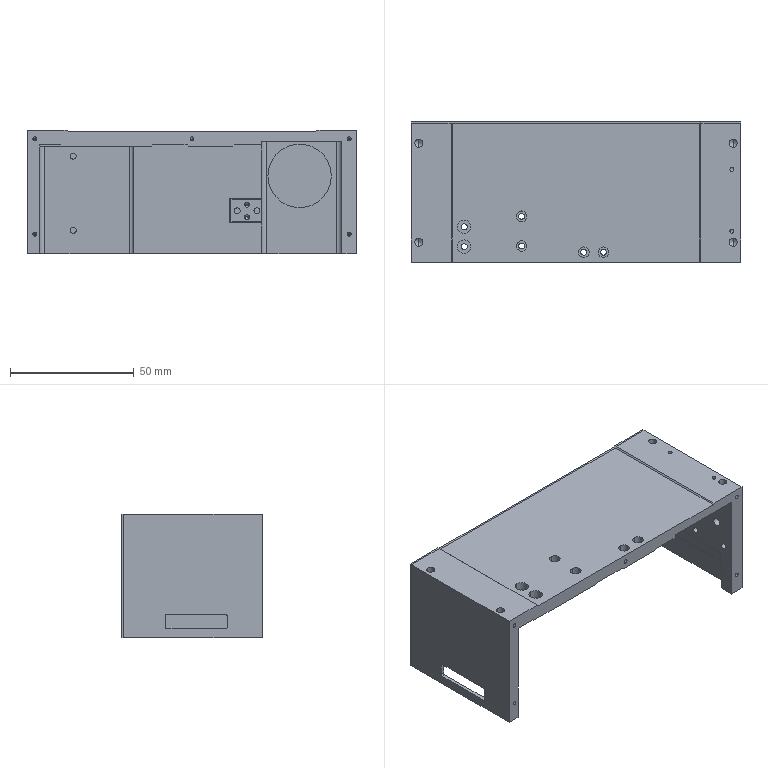NC program | NX | posted with a generic post | part box 133 x 56.74 x 50 mm
Whole program:
N10 G17 G21 G94 G90
(ZLEVEL_PROFILE_COPY , TOOL : D4)
N12 T04 M6
N14 G54
N16 G17 G0 G90 X1.724 Y-44.3 B0. C0. S9500 M3
N18 G43 Z30. H4
N20 Z1.5
N22 G94 G1 X12.07 Z0.958 F1000.
N24 Y-42.6 Z0.869
N26 X-8.53 Z-0.211
N28 Y-44.3 Z-0.3
N30 X12.07 F2000.
N32 Y-42.6
N34 X-8.53
N36 Y-44.3
N38 X8.657 Z-0.6
N40 X12.07
N42 Y-42.6
N44 X-8.53
N46 Y-44.3
N48 X8.657 Z-0.9
N50 X12.07
N52 Y-42.6
N54 X-8.53
N56 Y-44.3
N58 X8.657 Z-1.2
N60 X12.07
N62 Y-42.6
N64 X-8.53
N66 Y-44.3
N68 X8.657 Z-1.5
N70 X12.07
N72 Y-42.6
N74 X-8.53
N76 Y-44.3
N78 X8.657
N80 Z0.
N82 G0 Z30.
(ZLEVEL_PROFILE_COPY_COPY , TOOL : D4)
N84 X-8.63 Y-44.4
N86 Z3.
N88 G1 Z-1.5 F1000.
N90 X12.17
N92 Y-42.5
N94 X-8.63
N96 Y-44.4
N98 G3 X-8.284 Y-44.2 R0.4
N100 G1 Z1.5
N102 G0 Z30.
N104 M5
(ZLEVEL_PROFILE_COPY_COPY_1 , TOOL : D1)
N106 T01 M6
N108 G54
N110 G17 G0 G90 X11.925 Y-45.7 B0. C0. S9500 M3
N112 G43 Z30. H1
N114 Z0.921
N116 G94 G1 Z-0.079 F800.
N118 X12.012 Y-45.85
N120 X12.033 Y-45.913
N122 X12.098 Y-45.9
N124 X13.442
N126 X13.67 Y-45.885
N128 Y-44.328
N130 X13.683 Y-44.263
N132 X13.62 Y-44.242
N134 X13.47 Y-44.155
N136 Z0.921
N138 G0 X11.925 Y-45.7 Z0.842
N140 G1 Z-0.158
N142 X12.012 Y-45.85
N144 X12.033 Y-45.913
N146 X12.098 Y-45.9
N148 X13.442
N150 X13.67 Y-45.885
N152 Y-44.328
N154 X13.683 Y-44.263
N156 X13.62 Y-44.242
N158 X13.47 Y-44.155
N160 Z0.842
N162 G0 X11.925 Y-45.7 Z0.763
N164 G1 Z-0.237
N166 X12.012 Y-45.85
N168 X12.033 Y-45.913
N170 X12.098 Y-45.9
N172 X13.442
N174 X13.67 Y-45.885
N176 Y-44.328
N178 X13.683 Y-44.263
N180 X13.62 Y-44.242
N182 X13.47 Y-44.155
N184 Z0.763
N186 G0 X11.925 Y-45.7 Z0.684
N188 G1 Z-0.316
N190 X12.012 Y-45.85
N192 X12.033 Y-45.913
N194 X12.098 Y-45.9
N196 X13.442
N198 X13.67 Y-45.885
N200 Y-44.328
N202 X13.683 Y-44.263
N204 X13.62 Y-44.242
N206 X13.47 Y-44.155
N208 Z0.684
N210 G0 X11.925 Y-45.7 Z0.605
N212 G1 Z-0.395
N214 X12.012 Y-45.85
N216 X12.033 Y-45.913
N218 X12.098 Y-45.9
N220 X13.442
N222 X13.67 Y-45.885
N224 Y-44.328
N226 X13.683 Y-44.263
N228 X13.62 Y-44.242
N230 X13.47 Y-44.155
N232 Z0.605
N234 G0 X11.925 Y-45.7 Z0.526
N236 G1 Z-0.474
N238 X12.012 Y-45.85
N240 X12.033 Y-45.913
N242 X12.098 Y-45.9
N244 X13.442
N246 X13.67 Y-45.885
N248 Y-44.328
N250 X13.683 Y-44.263
N252 X13.62 Y-44.242
N254 X13.47 Y-44.155
N256 Z0.526
N258 G0 X11.925 Y-45.7 Z0.447
N260 G1 Z-0.553
N262 X12.012 Y-45.85
N264 X12.033 Y-45.913
N266 X12.098 Y-45.9
N268 X13.442
N270 X13.67 Y-45.885
N272 Y-44.328
N274 X13.683 Y-44.263
N276 X13.62 Y-44.242
N278 X13.47 Y-44.155
N280 Z0.447
N282 G0 X11.925 Y-45.7 Z0.368
N284 G1 Z-0.632
N286 X12.012 Y-45.85
N288 X12.033 Y-45.913
N290 X12.098 Y-45.9
N292 X13.442
N294 X13.67 Y-45.885
N296 Y-44.328
N298 X13.683 Y-44.263
N300 X13.62 Y-44.242
N302 X13.47 Y-44.155
N304 Z0.368
N306 G0 X11.925 Y-45.7 Z0.289
N308 G1 Z-0.711
N310 X12.012 Y-45.85
N312 X12.033 Y-45.913
N314 X12.098 Y-45.9
N316 X13.442
N318 X13.67 Y-45.885
N320 Y-44.328
N322 X13.683 Y-44.263
N324 X13.62 Y-44.242
N326 X13.47 Y-44.155
N328 Z0.289
N330 G0 X11.925 Y-45.7 Z0.211
N332 G1 Z-0.789
N334 X12.012 Y-45.85
N336 X12.033 Y-45.913
N338 X12.098 Y-45.9
N340 X13.442
N342 X13.67 Y-45.885
N344 Y-44.328
N346 X13.683 Y-44.263
N348 X13.62 Y-44.242
N350 X13.47 Y-44.155
N352 Z0.211
N354 G0 X11.925 Y-45.7 Z0.132
N356 G1 Z-0.868
N358 X12.012 Y-45.85
N360 X12.033 Y-45.913
N362 X12.098 Y-45.9
N364 X13.442
N366 X13.67 Y-45.885
N368 Y-44.328
N370 X13.683 Y-44.263
N372 X13.62 Y-44.242
N374 X13.47 Y-44.155
N376 Z0.132
N378 G0 X11.925 Y-45.7 Z0.053
N380 G1 Z-0.947
N382 X12.012 Y-45.85
N384 X12.033 Y-45.913
N386 X12.098 Y-45.9
N388 X13.442
N390 X13.67 Y-45.885
N392 Y-44.328
N394 X13.683 Y-44.263
N396 X13.62 Y-44.242
N398 X13.47 Y-44.155
N400 Z0.053
N402 G0 X11.925 Y-45.7 Z-0.026
N404 G1 Z-1.026
N406 X12.012 Y-45.85
N408 X12.033 Y-45.913
N410 X12.098 Y-45.9
N412 X13.442
N414 X13.67 Y-45.885
N416 Y-44.328
N418 X13.683 Y-44.263
N420 X13.62 Y-44.242
N422 X13.47 Y-44.155
N424 Z-0.026
N426 G0 X11.925 Y-45.7 Z-0.105
N428 G1 Z-1.105
N430 X12.011 Y-45.85
N432 X12.033 Y-45.913
N434 X12.098 Y-45.9
N436 X13.442
N438 X13.67 Y-45.885
N440 Y-44.328
N442 X13.683 Y-44.263
N444 X13.62 Y-44.241
N446 X13.47 Y-44.155
N448 Z-0.105
N450 G0 X11.925 Y-45.7 Z-0.184
N452 G1 Z-1.184
N454 X12.011 Y-45.85
N456 X12.033 Y-45.913
N458 X12.098 Y-45.9
N460 X13.442
N462 X13.67 Y-45.885
N464 Y-44.328
N466 X13.683 Y-44.263
N468 X13.62 Y-44.241
N470 X13.47 Y-44.155
N472 Z-0.184
N474 G0 X11.925 Y-45.7 Z-0.263
N476 G1 Z-1.263
N478 X12.011 Y-45.85
N480 X12.033 Y-45.913
N482 X12.098 Y-45.9
N484 X13.442
N486 X13.67 Y-45.885
N488 Y-44.328
N490 X13.683 Y-44.263
N492 X13.62 Y-44.241
N494 X13.47 Y-44.155
N496 Z-0.263
N498 G0 X11.925 Y-45.7 Z-0.342
N500 G1 Z-1.342
N502 X12.011 Y-45.85
N504 X12.033 Y-45.913
N506 X12.098 Y-45.9
N508 X13.659
N510 X13.67 Y-45.885
N512 Y-44.328
N514 X13.683 Y-44.263
N516 X13.62 Y-44.241
N518 X13.47 Y-44.155
N520 Z-0.342
N522 G0 X11.925 Y-45.7 Z-0.421
N524 G1 Z-1.421
N526 X12.011 Y-45.85
N528 X12.033 Y-45.913
N530 X12.098 Y-45.9
N532 X13.658
N534 X13.67 Y-45.885
N536 Y-44.328
N538 X13.683 Y-44.263
N540 X13.62 Y-44.241
N542 X13.47 Y-44.155
N544 Z-0.421
N546 G0 X11.925 Y-45.7 Z-0.5
N548 G1 Z-1.5
N550 X12.011 Y-45.85
N552 X12.033 Y-45.913
N554 X12.098 Y-45.9
N556 X13.658
N558 X13.67 Y-45.885
N560 Y-44.328
N562 X13.683 Y-44.263
N564 X13.62 Y-44.241
N566 X13.47 Y-44.155
N568 Z-0.5
N570 G0 Z30.
N572 Y-42.745
N574 Z0.921
N576 G1 Z-0.079
N578 X13.62 Y-42.658
N580 X13.683 Y-42.637
N582 X13.67 Y-42.572
N584 Y-41.
N586 X12.098
N588 X12.033 Y-40.987
N590 X12.012 Y-41.05
N592 X11.925 Y-41.2
N594 Z0.921
N596 G0 X13.47 Y-42.745 Z0.842
N598 G1 Z-0.158
N600 X13.62 Y-42.658
N602 X13.683 Y-42.637
N604 X13.67 Y-42.572
N606 Y-41.
N608 X12.098
N610 X12.033 Y-40.987
N612 X12.012 Y-41.05
N614 X11.925 Y-41.2
N616 Z0.842
N618 G0 X13.47 Y-42.745 Z0.763
N620 G1 Z-0.237
N622 X13.62 Y-42.658
N624 X13.683 Y-42.637
N626 X13.67 Y-42.572
N628 Y-41.
N630 X12.098
N632 X12.033 Y-40.987
N634 X12.012 Y-41.05
N636 X11.925 Y-41.2
N638 Z0.763
N640 G0 X13.47 Y-42.745 Z0.684
N642 G1 Z-0.316
N644 X13.62 Y-42.658
N646 X13.683 Y-42.637
N648 X13.67 Y-42.572
N650 Y-41.
N652 X12.098
N654 X12.033 Y-40.987
N656 X12.012 Y-41.05
N658 X11.925 Y-41.2
N660 Z0.684
N662 G0 X13.47 Y-42.745 Z0.605
N664 G1 Z-0.395
N666 X13.62 Y-42.658
N668 X13.683 Y-42.637
N670 X13.67 Y-42.572
N672 Y-41.
N674 X12.098
N676 X12.033 Y-40.987
N678 X12.012 Y-41.05
N680 X11.925 Y-41.2
N682 Z0.605
N684 G0 X13.47 Y-42.745 Z0.526
N686 G1 Z-0.474
N688 X13.62 Y-42.658
N690 X13.683 Y-42.637
N692 X13.67 Y-42.572
N694 Y-41.
N696 X12.098
N698 X12.033 Y-40.987
N700 X12.012 Y-41.05
N702 X11.925 Y-41.2
N704 Z0.526
N706 G0 X13.47 Y-42.745 Z0.447
N708 G1 Z-0.553
N710 X13.62 Y-42.658
N712 X13.683 Y-42.637
N714 X13.67 Y-42.572
N716 Y-41.
N718 X12.098
N720 X12.033 Y-40.987
N722 X12.012 Y-41.05
N724 X11.925 Y-41.2
N726 Z0.447
N728 G0 X13.47 Y-42.745 Z0.368
N730 G1 Z-0.632
N732 X13.62 Y-42.658
N734 X13.683 Y-42.637
N736 X13.67 Y-42.572
N738 Y-41.
N740 X12.098
N742 X12.033 Y-40.987
N744 X12.012 Y-41.05
N746 X11.925 Y-41.2
N748 Z0.368
N750 G0 X13.47 Y-42.745 Z0.289
N752 G1 Z-0.711
N754 X13.62 Y-42.658
N756 X13.683 Y-42.637
N758 X13.67 Y-42.572
N760 Y-41.
N762 X12.098
N764 X12.033 Y-40.987
N766 X12.012 Y-41.05
N768 X11.925 Y-41.2
N770 Z0.289
N772 G0 X13.47 Y-42.745 Z0.211
N774 G1 Z-0.789
N776 X13.62 Y-42.658
N778 X13.683 Y-42.637
N780 X13.67 Y-42.572
N782 Y-41.
N784 X12.098
N786 X12.033 Y-40.987
N788 X12.012 Y-41.05
N790 X11.925 Y-41.2
N792 Z0.211
N794 G0 X13.47 Y-42.745 Z0.132
N796 G1 Z-0.868
N798 X13.62 Y-42.658
N800 X13.683 Y-42.637
N802 X13.67 Y-42.572
N804 Y-41.
N806 X12.098
N808 X12.033 Y-40.987
N810 X12.012 Y-41.05
N812 X11.925 Y-41.2
N814 Z0.132
N816 G0 X13.47 Y-42.745 Z0.053
N818 G1 Z-0.947
N820 X13.62 Y-42.658
N822 X13.683 Y-42.637
N824 X13.67 Y-42.572
N826 Y-41.
N828 X12.098
N830 X12.033 Y-40.987
N832 X12.012 Y-41.05
N834 X11.925 Y-41.2
N836 Z0.053
N838 G0 X13.47 Y-42.745 Z-0.026
N840 G1 Z-1.026
N842 X13.62 Y-42.658
N844 X13.683 Y-42.637
N846 X13.67 Y-42.572
N848 Y-41.
N850 X12.098
N852 X12.033 Y-40.987
N854 X12.012 Y-41.05
N856 X11.925 Y-41.2
N858 Z-0.026
N860 G0 X13.47 Y-42.745 Z-0.105
N862 G1 Z-1.105
N864 X13.62 Y-42.658
N866 X13.683 Y-42.637
N868 X13.67 Y-42.572
N870 Y-41.
N872 X12.098
N874 X12.033 Y-40.987
N876 X12.012 Y-41.05
N878 X11.925 Y-41.2
N880 Z-0.105
N882 G0 X13.47 Y-42.745 Z-0.184
N884 G1 Z-1.184
N886 X13.62 Y-42.658
N888 X13.683 Y-42.637
N890 X13.67 Y-42.572
N892 Y-41.
N894 X12.098
N896 X12.033 Y-40.987
N898 X12.012 Y-41.05
N900 X11.925 Y-41.2
N902 Z-0.184
N904 G0 X13.47 Y-42.745 Z-0.263
N906 G1 Z-1.263
N908 X13.62 Y-42.658
N910 X13.683 Y-42.637
N912 X13.67 Y-42.572
N914 Y-41.
N916 X12.098
N918 X12.033 Y-40.987
N920 X12.012 Y-41.05
N922 X11.925 Y-41.2
N924 Z-0.263
N926 G0 X13.47 Y-42.745 Z-0.342
N928 G1 Z-1.342
N930 X13.62 Y-42.658
N932 X13.683 Y-42.637
N934 X13.67 Y-42.572
N936 Y-41.
N938 X12.098
N940 X12.033 Y-40.987
N942 X12.012 Y-41.05
N944 X11.925 Y-41.2
N946 Z-0.342
N948 G0 X13.47 Y-42.745 Z-0.421
N950 G1 Z-1.421
N952 X13.62 Y-42.658
N954 X13.683 Y-42.637
N956 X13.67 Y-42.572
N958 Y-41.
N960 X12.098
N962 X12.033 Y-40.987
N964 X12.012 Y-41.05
N966 X11.925 Y-41.2
N968 Z-0.421
N970 G0 X13.47 Y-42.745 Z-0.5
N972 G1 Z-1.5
N974 X13.62 Y-42.658
N976 X13.683 Y-42.637
N978 X13.67 Y-42.572
N980 Y-41.
N982 X12.098
N984 X12.033 Y-40.987
N986 X12.012 Y-41.05
N988 X11.925 Y-41.2
N990 Z-0.5
N992 G0 Z30.
N994 X-8.385
N996 Z0.921
N998 G1 Z-0.079
N1000 X-8.472 Y-41.05
N1002 X-8.493 Y-40.987
N1004 X-8.558 Y-41.
N1006 X-10.13
N1008 Y-42.572
N1010 X-10.143 Y-42.637
N1012 X-10.08 Y-42.658
N1014 X-9.93 Y-42.745
N1016 Z0.921
N1018 G0 X-8.385 Y-41.2 Z0.842
N1020 G1 Z-0.158
N1022 X-8.472 Y-41.05
N1024 X-8.493 Y-40.987
N1026 X-8.558 Y-41.
N1028 X-10.13
N1030 Y-42.572
N1032 X-10.143 Y-42.637
N1034 X-10.08 Y-42.658
N1036 X-9.93 Y-42.745
N1038 Z0.842
N1040 G0 X-8.385 Y-41.2 Z0.763
N1042 G1 Z-0.237
N1044 X-8.472 Y-41.05
N1046 X-8.493 Y-40.987
N1048 X-8.558 Y-41.
N1050 X-10.13
N1052 Y-42.572
N1054 X-10.143 Y-42.637
N1056 X-10.08 Y-42.658
N1058 X-9.93 Y-42.745
N1060 Z0.763
N1062 G0 X-8.385 Y-41.2 Z0.684
N1064 G1 Z-0.316
N1066 X-8.472 Y-41.05
N1068 X-8.493 Y-40.987
N1070 X-8.558 Y-41.
N1072 X-10.13
N1074 Y-42.572
N1076 X-10.143 Y-42.637
N1078 X-10.08 Y-42.658
N1080 X-9.93 Y-42.745
N1082 Z0.684
N1084 G0 X-8.385 Y-41.2 Z0.605
N1086 G1 Z-0.395
N1088 X-8.472 Y-41.05
N1090 X-8.493 Y-40.987
N1092 X-8.558 Y-41.
N1094 X-10.13
N1096 Y-42.572
N1098 X-10.143 Y-42.637
N1100 X-10.08 Y-42.658
N1102 X-9.93 Y-42.745
N1104 Z0.605
N1106 G0 X-8.385 Y-41.2 Z0.526
N1108 G1 Z-0.474
N1110 X-8.472 Y-41.05
N1112 X-8.493 Y-40.987
N1114 X-8.558 Y-41.
N1116 X-10.13
N1118 Y-42.572
N1120 X-10.143 Y-42.637
N1122 X-10.08 Y-42.658
N1124 X-9.93 Y-42.745
N1126 Z0.526
N1128 G0 X-8.385 Y-41.2 Z0.447
N1130 G1 Z-0.553
N1132 X-8.472 Y-41.05
N1134 X-8.493 Y-40.987
N1136 X-8.558 Y-41.
N1138 X-10.13
N1140 Y-42.572
N1142 X-10.143 Y-42.637
N1144 X-10.08 Y-42.658
N1146 X-9.93 Y-42.745
N1148 Z0.447
N1150 G0 X-8.385 Y-41.2 Z0.368
N1152 G1 Z-0.632
N1154 X-8.472 Y-41.05
N1156 X-8.493 Y-40.987
N1158 X-8.558 Y-41.
N1160 X-10.13
N1162 Y-42.572
N1164 X-10.143 Y-42.637
N1166 X-10.08 Y-42.658
N1168 X-9.93 Y-42.745
N1170 Z0.368
N1172 G0 X-8.385 Y-41.2 Z0.289
N1174 G1 Z-0.711
N1176 X-8.472 Y-41.05
N1178 X-8.493 Y-40.987
N1180 X-8.558 Y-41.
N1182 X-10.13
N1184 Y-42.572
N1186 X-10.143 Y-42.637
N1188 X-10.08 Y-42.658
N1190 X-9.93 Y-42.745
N1192 Z0.289
N1194 G0 X-8.385 Y-41.2 Z0.211
N1196 G1 Z-0.789
N1198 X-8.472 Y-41.05
N1200 X-8.493 Y-40.987
N1202 X-8.558 Y-41.
N1204 X-10.13
N1206 Y-42.572
N1208 X-10.143 Y-42.637
N1210 X-10.08 Y-42.658
N1212 X-9.93 Y-42.745
N1214 Z0.211
N1216 G0 X-8.385 Y-41.2 Z0.132
N1218 G1 Z-0.868
N1220 X-8.472 Y-41.05
N1222 X-8.493 Y-40.987
N1224 X-8.558 Y-41.
N1226 X-10.13
N1228 Y-42.572
N1230 X-10.143 Y-42.637
N1232 X-10.08 Y-42.658
N1234 X-9.93 Y-42.745
N1236 Z0.132
N1238 G0 X-8.385 Y-41.2 Z0.053
N1240 G1 Z-0.947
N1242 X-8.472 Y-41.05
N1244 X-8.493 Y-40.987
N1246 X-8.558 Y-41.
N1248 X-10.13
N1250 Y-42.572
N1252 X-10.143 Y-42.637
N1254 X-10.08 Y-42.658
N1256 X-9.93 Y-42.745
N1258 Z0.053
N1260 G0 X-8.385 Y-41.2 Z-0.026
N1262 G1 Z-1.026
N1264 X-8.472 Y-41.05
N1266 X-8.493 Y-40.987
N1268 X-8.558 Y-41.
N1270 X-10.13
N1272 Y-42.572
N1274 X-10.143 Y-42.637
N1276 X-10.08 Y-42.658
N1278 X-9.93 Y-42.745
N1280 Z-0.026
N1282 G0 X-8.385 Y-41.2 Z-0.105
N1284 G1 Z-1.105
N1286 X-8.472 Y-41.05
N1288 X-8.493 Y-40.987
N1290 X-8.558 Y-41.
N1292 X-10.13
N1294 Y-42.572
N1296 X-10.143 Y-42.637
N1298 X-10.08 Y-42.658
N1300 X-9.93 Y-42.745
N1302 Z-0.105
N1304 G0 X-8.385 Y-41.2 Z-0.184
N1306 G1 Z-1.184
N1308 X-8.472 Y-41.05
N1310 X-8.493 Y-40.987
N1312 X-8.558 Y-41.
N1314 X-10.13
N1316 Y-42.572
N1318 X-10.143 Y-42.637
N1320 X-10.08 Y-42.658
N1322 X-9.93 Y-42.745
N1324 Z-0.184
N1326 G0 X-8.385 Y-41.2 Z-0.263
N1328 G1 Z-1.263
N1330 X-8.472 Y-41.05
N1332 X-8.493 Y-40.987
N1334 X-8.558 Y-41.
N1336 X-10.13
N1338 Y-42.572
N1340 X-10.143 Y-42.637
N1342 X-10.08 Y-42.658
N1344 X-9.93 Y-42.745
N1346 Z-0.263
N1348 G0 X-8.385 Y-41.2 Z-0.342
N1350 G1 Z-1.342
N1352 X-8.472 Y-41.05
N1354 X-8.493 Y-40.987
N1356 X-8.558 Y-41.
N1358 X-10.13
N1360 Y-42.572
N1362 X-10.143 Y-42.637
N1364 X-10.08 Y-42.658
N1366 X-9.93 Y-42.745
N1368 Z-0.342
N1370 G0 X-8.385 Y-41.2 Z-0.421
N1372 G1 Z-1.421
N1374 X-8.472 Y-41.05
N1376 X-8.493 Y-40.987
N1378 X-8.558 Y-41.
N1380 X-10.13
N1382 Y-42.572
N1384 X-10.143 Y-42.637
N1386 X-10.08 Y-42.658
N1388 X-9.93 Y-42.745
N1390 Z-0.421
N1392 G0 X-8.385 Y-41.2 Z-0.5
N1394 G1 Z-1.5
N1396 X-8.472 Y-41.05
N1398 X-8.493 Y-40.987
N1400 X-8.558 Y-41.
N1402 X-10.129
N1404 X-10.13 Y-42.572
N1406 X-10.143 Y-42.637
N1408 X-10.08 Y-42.658
N1410 X-9.93 Y-42.745
N1412 Z-0.5
N1414 G0 Z30.
N1416 Y-44.155
N1418 Z0.921
N1420 G1 Z-0.079
N1422 X-10.08 Y-44.242
N1424 X-10.143 Y-44.263
N1426 X-10.13 Y-44.328
N1428 Y-45.9
N1430 X-8.558
N1432 X-8.493 Y-45.913
N1434 X-8.472 Y-45.85
N1436 X-8.385 Y-45.7
N1438 Z0.921
N1440 G0 X-9.93 Y-44.155 Z0.842
N1442 G1 Z-0.158
N1444 X-10.08 Y-44.242
N1446 X-10.143 Y-44.263
N1448 X-10.13 Y-44.328
N1450 Y-45.9
N1452 X-8.558
N1454 X-8.493 Y-45.913
N1456 X-8.472 Y-45.85
N1458 X-8.385 Y-45.7
N1460 Z0.842
N1462 G0 X-9.93 Y-44.155 Z0.763
N1464 G1 Z-0.237
N1466 X-10.08 Y-44.242
N1468 X-10.143 Y-44.263
N1470 X-10.13 Y-44.328
N1472 Y-45.9
N1474 X-8.558
N1476 X-8.493 Y-45.913
N1478 X-8.472 Y-45.85
N1480 X-8.385 Y-45.7
N1482 Z0.763
N1484 G0 X-9.93 Y-44.155 Z0.684
N1486 G1 Z-0.316
N1488 X-10.08 Y-44.242
N1490 X-10.143 Y-44.263
N1492 X-10.13 Y-44.328
N1494 Y-45.9
N1496 X-8.558
N1498 X-8.493 Y-45.913
N1500 X-8.472 Y-45.85
N1502 X-8.385 Y-45.7
N1504 Z0.684
N1506 G0 X-9.93 Y-44.155 Z0.605
N1508 G1 Z-0.395
N1510 X-10.08 Y-44.242
N1512 X-10.143 Y-44.263
N1514 X-10.13 Y-44.328
N1516 Y-45.9
N1518 X-8.558
N1520 X-8.493 Y-45.913
N1522 X-8.472 Y-45.85
N1524 X-8.385 Y-45.7
N1526 Z0.605
N1528 G0 X-9.93 Y-44.155 Z0.526
N1530 G1 Z-0.474
N1532 X-10.08 Y-44.242
N1534 X-10.143 Y-44.263
N1536 X-10.13 Y-44.328
N1538 Y-45.9
N1540 X-8.558
N1542 X-8.493 Y-45.913
N1544 X-8.472 Y-45.85
N1546 X-8.385 Y-45.7
N1548 Z0.526
N1550 G0 X-9.93 Y-44.155 Z0.447
N1552 G1 Z-0.553
N1554 X-10.08 Y-44.242
N1556 X-10.143 Y-44.263
N1558 X-10.13 Y-44.328
N1560 Y-45.9
N1562 X-8.558
N1564 X-8.493 Y-45.913
N1566 X-8.472 Y-45.85
N1568 X-8.385 Y-45.7
N1570 Z0.447
N1572 G0 X-9.93 Y-44.155 Z0.368
N1574 G1 Z-0.632
N1576 X-10.08 Y-44.242
N1578 X-10.143 Y-44.263
N1580 X-10.13 Y-44.328
N1582 Y-45.9
N1584 X-8.558
N1586 X-8.493 Y-45.913
N1588 X-8.472 Y-45.85
N1590 X-8.385 Y-45.7
N1592 Z0.368
N1594 G0 X-9.93 Y-44.155 Z0.289
N1596 G1 Z-0.711
N1598 X-10.08 Y-44.242
N1600 X-10.143 Y-44.263
N1602 X-10.13 Y-44.328
N1604 Y-45.9
N1606 X-8.558
N1608 X-8.493 Y-45.913
N1610 X-8.472 Y-45.85
N1612 X-8.385 Y-45.7
N1614 Z0.289
N1616 G0 X-9.93 Y-44.155 Z0.211
N1618 G1 Z-0.789
N1620 X-10.08 Y-44.242
N1622 X-10.143 Y-44.263
N1624 X-10.13 Y-44.328
N1626 Y-45.9
N1628 X-8.558
N1630 X-8.493 Y-45.913
N1632 X-8.472 Y-45.85
N1634 X-8.385 Y-45.7
N1636 Z0.211
N1638 G0 X-9.93 Y-44.155 Z0.132
N1640 G1 Z-0.868
N1642 X-10.08 Y-44.242
N1644 X-10.143 Y-44.263
N1646 X-10.13 Y-44.328
N1648 Y-45.9
N1650 X-8.558
N1652 X-8.493 Y-45.913
N1654 X-8.472 Y-45.85
N1656 X-8.385 Y-45.7
N1658 Z0.132
N1660 G0 X-9.93 Y-44.155 Z0.053
N1662 G1 Z-0.947
N1664 X-10.08 Y-44.242
N1666 X-10.143 Y-44.263
N1668 X-10.13 Y-44.328
N1670 Y-45.9
N1672 X-8.558
N1674 X-8.493 Y-45.913
N1676 X-8.472 Y-45.85
N1678 X-8.385 Y-45.7
N1680 Z0.053
N1682 G0 X-9.93 Y-44.155 Z-0.026
N1684 G1 Z-1.026
N1686 X-10.08 Y-44.242
N1688 X-10.143 Y-44.263
N1690 X-10.13 Y-44.328
N1692 Y-45.9
N1694 X-8.558
N1696 X-8.493 Y-45.913
N1698 X-8.472 Y-45.85
N1700 X-8.385 Y-45.7
N1702 Z-0.026
N1704 G0 X-9.93 Y-44.155 Z-0.105
N1706 G1 Z-1.105
N1708 X-10.08 Y-44.242
N1710 X-10.143 Y-44.263
N1712 X-10.13 Y-44.328
N1714 Y-45.9
N1716 X-8.558
N1718 X-8.493 Y-45.913
N1720 X-8.472 Y-45.85
N1722 X-8.385 Y-45.7
N1724 Z-0.105
N1726 G0 X-9.93 Y-44.155 Z-0.184
N1728 G1 Z-1.184
N1730 X-10.08 Y-44.242
N1732 X-10.143 Y-44.263
N1734 X-10.13 Y-44.328
N1736 Y-45.9
N1738 X-8.558
N1740 X-8.493 Y-45.913
N1742 X-8.472 Y-45.85
N1744 X-8.385 Y-45.7
N1746 Z-0.184
N1748 G0 X-9.93 Y-44.155 Z-0.263
N1750 G1 Z-1.263
N1752 X-10.08 Y-44.242
N1754 X-10.143 Y-44.263
N1756 X-10.13 Y-44.328
N1758 Y-45.9
N1760 X-8.558
N1762 X-8.493 Y-45.913
N1764 X-8.472 Y-45.85
N1766 X-8.385 Y-45.7
N1768 Z-0.263
N1770 G0 X-9.93 Y-44.155 Z-0.342
N1772 G1 Z-1.342
N1774 X-10.08 Y-44.242
N1776 X-10.143 Y-44.263
N1778 X-10.13 Y-44.328
N1780 Y-45.9
N1782 X-8.558
N1784 X-8.493 Y-45.913
N1786 X-8.472 Y-45.85
N1788 X-8.385 Y-45.7
N1790 Z-0.342
N1792 G0 X-9.93 Y-44.155 Z-0.421
N1794 G1 Z-1.421
N1796 X-10.08 Y-44.242
N1798 X-10.143 Y-44.263
N1800 X-10.13 Y-44.328
N1802 Y-45.9
N1804 X-8.558
N1806 X-8.493 Y-45.913
N1808 X-8.472 Y-45.85
N1810 X-8.385 Y-45.7
N1812 Z-0.421
N1814 G0 X-9.93 Y-44.155 Z-0.5
N1816 G1 Z-1.5
N1818 X-10.08 Y-44.242
N1820 X-10.143 Y-44.263
N1822 X-10.13 Y-44.328
N1824 Y-45.9
N1826 X-8.558
N1828 X-8.493 Y-45.913
N1830 X-8.472 Y-45.85
N1832 X-8.385 Y-45.7
N1834 Z-0.5
N1836 G0 Z30.
N1838 M5
(PLANAR_MILL_COPY_1_COPY , TOOL : D6A45)
N1840 T07 M6
N1842 G54
N1844 G17 G0 G90 X-8.53 Y-44.23 B0. C0. S9500 M3
N1846 G43 Z30. H7
N1848 Z0.5
N1850 G94 G1 Z-1. F1250.
N1852 X-9.23 Y-44.634
N1854 G3 X-9.73 Y-45.5 R1.
N1856 G1 X13.27
N1858 Y-41.4
N1860 X-9.73
N1862 Y-45.5
N1864 G3 X-8.864 Y-45. R1.
N1866 G1 X-8.46 Y-44.3
N1868 Z0.5
N1870 G0 Z30.
N1872 M5
N1874 M2